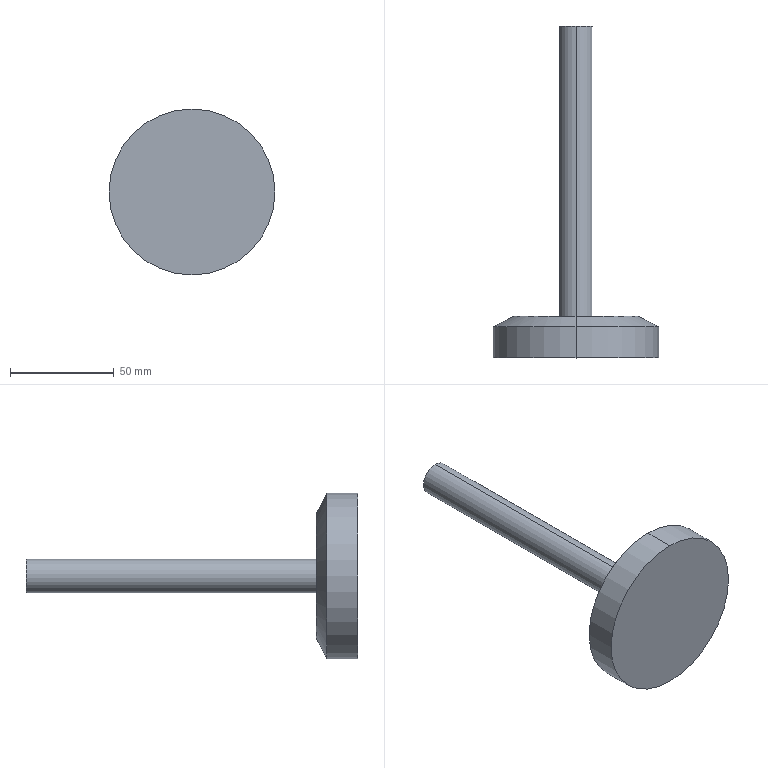Part | SolidWorks | features Revolution 1 | 1 solid | 9 faces | box 80 x 160 x 80 mm | volume 122920 mm3 | cylinder 4 | plane 3 | cone 2 | commonest cylinder face diameters 16 x2 80 x2
STEP:
#1=CARTESIAN_POINT('',(0.,160.,-8.));
#2=VERTEX_POINT('',#1);
#3=CARTESIAN_POINT('',(0.,160.,8.));
#4=VERTEX_POINT('',#3);
#5=CARTESIAN_POINT('',(0.,160.,0.));
#6=DIRECTION('',(0.,-1.,0.));
#7=DIRECTION('',(0.,0.,-1.));
#8=AXIS2_PLACEMENT_3D('',#5,#6,#7);
#9=CIRCLE('',#8,8.);
#10=EDGE_CURVE('',#2,#4,#9,.T.);
#11=ORIENTED_EDGE('',*,*,#10,.T.);
#12=CARTESIAN_POINT('',(0.,20.,8.));
#13=VERTEX_POINT('',#12);
#14=CARTESIAN_POINT('',(0.,0.,8.));
#15=DIRECTION('',(0.,-1.,0.));
#16=VECTOR('',#15,1000.);
#17=LINE('',#14,#16);
#18=EDGE_CURVE('',#4,#13,#17,.T.);
#19=ORIENTED_EDGE('',*,*,#18,.T.);
#20=CARTESIAN_POINT('',(0.,20.,-8.));
#21=VERTEX_POINT('',#20);
#22=CARTESIAN_POINT('',(0.,20.,0.));
#23=DIRECTION('',(0.,-1.,0.));
#24=DIRECTION('',(0.,0.,-1.));
#25=AXIS2_PLACEMENT_3D('',#22,#23,#24);
#26=CIRCLE('',#25,8.);
#27=EDGE_CURVE('',#21,#13,#26,.T.);
#28=ORIENTED_EDGE('',*,*,#27,.F.);
#29=CARTESIAN_POINT('',(0.,0.,-8.));
#30=DIRECTION('',(0.,-1.,0.));
#31=VECTOR('',#30,1000.);
#32=LINE('',#29,#31);
#33=EDGE_CURVE('',#2,#21,#32,.T.);
#34=ORIENTED_EDGE('',*,*,#33,.F.);
#35=EDGE_LOOP('',(#11,#19,#28,#34));
#36=FACE_OUTER_BOUND('',#35,.T.);
#37=CARTESIAN_POINT('',(0.,0.,0.));
#38=DIRECTION('',(0.,-1.,0.));
#39=DIRECTION('',(0.,0.,-1.));
#40=AXIS2_PLACEMENT_3D('',#37,#38,#39);
#41=CYLINDRICAL_SURFACE('',#40,8.);
#42=ADVANCED_FACE('',(#36),#41,.T.);
#43=CARTESIAN_POINT('',(0.,20.,-30.));
#44=VERTEX_POINT('',#43);
#45=CARTESIAN_POINT('',(0.,20.,30.));
#46=VERTEX_POINT('',#45);
#47=CARTESIAN_POINT('',(0.,20.,0.));
#48=DIRECTION('',(0.,-1.,0.));
#49=DIRECTION('',(0.,0.,-1.));
#50=AXIS2_PLACEMENT_3D('',#47,#48,#49);
#51=CIRCLE('',#50,30.);
#52=EDGE_CURVE('',#44,#46,#51,.T.);
#53=ORIENTED_EDGE('',*,*,#52,.T.);
#54=CARTESIAN_POINT('',(0.,15.,40.));
#55=VERTEX_POINT('',#54);
#56=CARTESIAN_POINT('',(0.,15.,40.));
#57=DIRECTION('',(0.,-0.4472,0.8944));
#58=VECTOR('',#57,1000.);
#59=LINE('',#56,#58);
#60=EDGE_CURVE('',#46,#55,#59,.T.);
#61=ORIENTED_EDGE('',*,*,#60,.T.);
#62=CARTESIAN_POINT('',(0.,15.,-40.));
#63=VERTEX_POINT('',#62);
#64=CARTESIAN_POINT('',(0.,15.,0.));
#65=DIRECTION('',(0.,-1.,0.));
#66=DIRECTION('',(0.,0.,-1.));
#67=AXIS2_PLACEMENT_3D('',#64,#65,#66);
#68=CIRCLE('',#67,40.);
#69=EDGE_CURVE('',#63,#55,#68,.T.);
#70=ORIENTED_EDGE('',*,*,#69,.F.);
#71=CARTESIAN_POINT('',(0.,15.,-40.));
#72=DIRECTION('',(0.,-0.4472,-0.8944));
#73=VECTOR('',#72,1000.);
#74=LINE('',#71,#73);
#75=EDGE_CURVE('',#44,#63,#74,.T.);
#76=ORIENTED_EDGE('',*,*,#75,.F.);
#77=EDGE_LOOP('',(#53,#61,#70,#76));
#78=FACE_OUTER_BOUND('',#77,.T.);
#79=CARTESIAN_POINT('',(0.,15.,0.));
#80=DIRECTION('',(0.,-1.,0.));
#81=DIRECTION('',(0.,0.,-1.));
#82=AXIS2_PLACEMENT_3D('',#79,#80,#81);
#83=CONICAL_SURFACE('',#82,40.,1.107);
#84=ADVANCED_FACE('',(#78),#83,.T.);
#85=ORIENTED_EDGE('',*,*,#69,.T.);
#86=CARTESIAN_POINT('',(0.,0.,40.));
#87=VERTEX_POINT('',#86);
#88=CARTESIAN_POINT('',(0.,0.,40.));
#89=DIRECTION('',(0.,-1.,0.));
#90=VECTOR('',#89,1000.);
#91=LINE('',#88,#90);
#92=EDGE_CURVE('',#55,#87,#91,.T.);
#93=ORIENTED_EDGE('',*,*,#92,.T.);
#94=CARTESIAN_POINT('',(0.,0.,-40.));
#95=VERTEX_POINT('',#94);
#96=CARTESIAN_POINT('',(0.,0.,0.));
#97=DIRECTION('',(0.,-1.,0.));
#98=DIRECTION('',(0.,0.,-1.));
#99=AXIS2_PLACEMENT_3D('',#96,#97,#98);
#100=CIRCLE('',#99,40.);
#101=EDGE_CURVE('',#95,#87,#100,.T.);
#102=ORIENTED_EDGE('',*,*,#101,.F.);
#103=CARTESIAN_POINT('',(0.,0.,-40.));
#104=DIRECTION('',(0.,-1.,0.));
#105=VECTOR('',#104,1000.);
#106=LINE('',#103,#105);
#107=EDGE_CURVE('',#63,#95,#106,.T.);
#108=ORIENTED_EDGE('',*,*,#107,.F.);
#109=EDGE_LOOP('',(#85,#93,#102,#108));
#110=FACE_OUTER_BOUND('',#109,.T.);
#111=CARTESIAN_POINT('',(0.,0.,0.));
#112=DIRECTION('',(0.,-1.,0.));
#113=DIRECTION('',(0.,0.,-1.));
#114=AXIS2_PLACEMENT_3D('',#111,#112,#113);
#115=CYLINDRICAL_SURFACE('',#114,40.);
#116=ADVANCED_FACE('',(#110),#115,.T.);
#117=ORIENTED_EDGE('',*,*,#101,.T.);
#118=CARTESIAN_POINT('',(0.,0.,0.));
#119=DIRECTION('',(0.,-1.,0.));
#120=DIRECTION('',(0.,0.,-1.));
#121=AXIS2_PLACEMENT_3D('',#118,#119,#120);
#122=CIRCLE('',#121,40.);
#123=EDGE_CURVE('',#87,#95,#122,.T.);
#124=ORIENTED_EDGE('',*,*,#123,.T.);
#125=EDGE_LOOP('',(#117,#124));
#126=FACE_OUTER_BOUND('',#125,.T.);
#127=CARTESIAN_POINT('',(0.,0.,0.));
#128=DIRECTION('',(0.,-1.,0.));
#129=DIRECTION('',(0.,0.,-1.));
#130=AXIS2_PLACEMENT_3D('',#127,#128,#129);
#131=PLANE('',#130);
#132=ADVANCED_FACE('',(#126),#131,.T.);
#133=ORIENTED_EDGE('',*,*,#92,.F.);
#134=CARTESIAN_POINT('',(0.,15.,0.));
#135=DIRECTION('',(0.,-1.,0.));
#136=DIRECTION('',(0.,0.,-1.));
#137=AXIS2_PLACEMENT_3D('',#134,#135,#136);
#138=CIRCLE('',#137,40.);
#139=EDGE_CURVE('',#55,#63,#138,.T.);
#140=ORIENTED_EDGE('',*,*,#139,.T.);
#141=ORIENTED_EDGE('',*,*,#107,.T.);
#142=ORIENTED_EDGE('',*,*,#123,.F.);
#143=EDGE_LOOP('',(#133,#140,#141,#142));
#144=FACE_OUTER_BOUND('',#143,.T.);
#145=CARTESIAN_POINT('',(0.,0.,0.));
#146=DIRECTION('',(0.,-1.,0.));
#147=DIRECTION('',(0.,0.,-1.));
#148=AXIS2_PLACEMENT_3D('',#145,#146,#147);
#149=CYLINDRICAL_SURFACE('',#148,40.);
#150=ADVANCED_FACE('',(#144),#149,.T.);
#151=ORIENTED_EDGE('',*,*,#60,.F.);
#152=CARTESIAN_POINT('',(0.,20.,0.));
#153=DIRECTION('',(0.,-1.,0.));
#154=DIRECTION('',(0.,0.,-1.));
#155=AXIS2_PLACEMENT_3D('',#152,#153,#154);
#156=CIRCLE('',#155,30.);
#157=EDGE_CURVE('',#46,#44,#156,.T.);
#158=ORIENTED_EDGE('',*,*,#157,.T.);
#159=ORIENTED_EDGE('',*,*,#75,.T.);
#160=ORIENTED_EDGE('',*,*,#139,.F.);
#161=EDGE_LOOP('',(#151,#158,#159,#160));
#162=FACE_OUTER_BOUND('',#161,.T.);
#163=CARTESIAN_POINT('',(0.,15.,0.));
#164=DIRECTION('',(0.,-1.,0.));
#165=DIRECTION('',(0.,0.,-1.));
#166=AXIS2_PLACEMENT_3D('',#163,#164,#165);
#167=CONICAL_SURFACE('',#166,40.,1.107);
#168=ADVANCED_FACE('',(#162),#167,.T.);
#169=ORIENTED_EDGE('',*,*,#27,.T.);
#170=CARTESIAN_POINT('',(0.,20.,0.));
#171=DIRECTION('',(0.,-1.,0.));
#172=DIRECTION('',(0.,0.,-1.));
#173=AXIS2_PLACEMENT_3D('',#170,#171,#172);
#174=CIRCLE('',#173,8.);
#175=EDGE_CURVE('',#13,#21,#174,.T.);
#176=ORIENTED_EDGE('',*,*,#175,.T.);
#177=EDGE_LOOP('',(#169,#176));
#178=FACE_BOUND('',#177,.T.);
#179=ORIENTED_EDGE('',*,*,#52,.F.);
#180=ORIENTED_EDGE('',*,*,#157,.F.);
#181=EDGE_LOOP('',(#179,#180));
#182=FACE_OUTER_BOUND('',#181,.T.);
#183=CARTESIAN_POINT('',(30.,20.,0.));
#184=DIRECTION('',(0.,1.,0.));
#185=DIRECTION('',(0.,0.,1.));
#186=AXIS2_PLACEMENT_3D('',#183,#184,#185);
#187=PLANE('',#186);
#188=ADVANCED_FACE('',(#178,#182),#187,.T.);
#189=ORIENTED_EDGE('',*,*,#18,.F.);
#190=CARTESIAN_POINT('',(0.,160.,0.));
#191=DIRECTION('',(0.,-1.,0.));
#192=DIRECTION('',(0.,0.,-1.));
#193=AXIS2_PLACEMENT_3D('',#190,#191,#192);
#194=CIRCLE('',#193,8.);
#195=EDGE_CURVE('',#4,#2,#194,.T.);
#196=ORIENTED_EDGE('',*,*,#195,.T.);
#197=ORIENTED_EDGE('',*,*,#33,.T.);
#198=ORIENTED_EDGE('',*,*,#175,.F.);
#199=EDGE_LOOP('',(#189,#196,#197,#198));
#200=FACE_OUTER_BOUND('',#199,.T.);
#201=CARTESIAN_POINT('',(0.,0.,0.));
#202=DIRECTION('',(0.,-1.,0.));
#203=DIRECTION('',(0.,0.,-1.));
#204=AXIS2_PLACEMENT_3D('',#201,#202,#203);
#205=CYLINDRICAL_SURFACE('',#204,8.);
#206=ADVANCED_FACE('',(#200),#205,.T.);
#207=ORIENTED_EDGE('',*,*,#10,.F.);
#208=ORIENTED_EDGE('',*,*,#195,.F.);
#209=EDGE_LOOP('',(#207,#208));
#210=FACE_OUTER_BOUND('',#209,.T.);
#211=CARTESIAN_POINT('',(8.,160.,0.));
#212=DIRECTION('',(0.,1.,0.));
#213=DIRECTION('',(0.,0.,1.));
#214=AXIS2_PLACEMENT_3D('',#211,#212,#213);
#215=PLANE('',#214);
#216=ADVANCED_FACE('',(#210),#215,.T.);
#217=CLOSED_SHELL('',(#42,#84,#116,#132,#150,#168,#188,#206,#216));
#218=MANIFOLD_SOLID_BREP('',#217);
#219=CARTESIAN_POINT('',(0.,0.,0.));
#220=DIRECTION('',(0.,0.,1.));
#221=DIRECTION('',(1.,0.,0.));
#222=AXIS2_PLACEMENT_3D('',#219,#220,#221);
#223=(LENGTH_UNIT()NAMED_UNIT(*)SI_UNIT(.MILLI.,.METRE.));
#224=UNCERTAINTY_MEASURE_WITH_UNIT(LENGTH_MEASURE(0.00001),#223,'','');
#225=(NAMED_UNIT(*)PLANE_ANGLE_UNIT()SI_UNIT($,.RADIAN.));
#226=(NAMED_UNIT(*)SI_UNIT($,.STERADIAN.)SOLID_ANGLE_UNIT());
#227=(GEOMETRIC_REPRESENTATION_CONTEXT(3)GLOBAL_UNCERTAINTY_ASSIGNED_CONTEXT((#224))GLOBAL_UNIT_ASSIGNED_CONTEXT((#223,#225,#226))REPRESENTATION_CONTEXT('',''));
#228=ADVANCED_BREP_SHAPE_REPRESENTATION('',(#218,#222),#227);